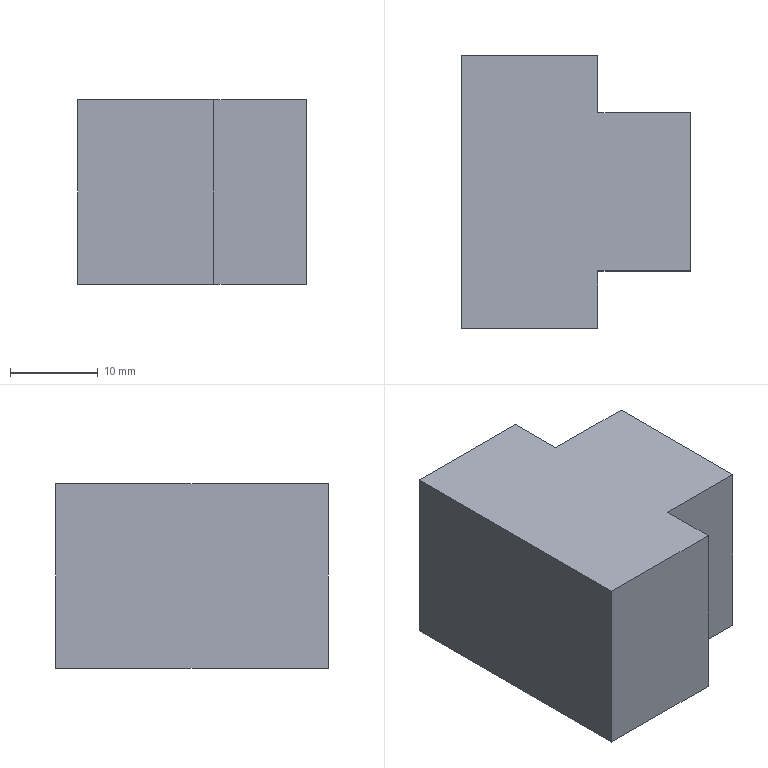Part | STEP file | PN_0024 | 1 solid | 13 faces | box 26 x 31 x 21 mm | volume 12363 mm3 | plane 11 | cylinder 2 | commonest cylinder face diameters 12 x2
STEP:
#1=CARTESIAN_POINT('',(0.,0.,0.));
#2=DIRECTION('',(0.,0.,1.));
#3=DIRECTION('',(1.,0.,0.));
#4=AXIS2_PLACEMENT_3D('',#1,#2,#3);
#5=CARTESIAN_POINT('',(11.,15.5,4.5));
#6=VERTEX_POINT('',#5);
#7=CARTESIAN_POINT('',(26.,15.5,4.5));
#8=VERTEX_POINT('',#7);
#9=CARTESIAN_POINT('',(11.,15.5,4.5));
#10=DIRECTION('',(1.,0.,0.));
#11=VECTOR('',#10,1.);
#12=LINE('',#9,#11);
#13=CARTESIAN_POINT('',(11.,15.5,10.5));
#14=DIRECTION('',(1.,0.,0.));
#15=DIRECTION('',(0.,0.,-1.));
#16=AXIS2_PLACEMENT_3D('',#13,#14,#15);
#17=CYLINDRICAL_SURFACE('',#16,6.);
#18=CARTESIAN_POINT('',(6.283,0.));
#19=DIRECTION('',(0.,1.));
#20=VECTOR('',#19,1.);
#21=LINE('',#18,#20);
#22=(GEOMETRIC_REPRESENTATION_CONTEXT(2)PARAMETRIC_REPRESENTATION_CONTEXT()REPRESENTATION_CONTEXT('',''));
#23=DEFINITIONAL_REPRESENTATION('',(#21),#22);
#24=PCURVE('',#17,#23);
#25=CARTESIAN_POINT('',(11.,15.5,10.5));
#26=DIRECTION('',(1.,0.,0.));
#27=DIRECTION('',(0.,0.,-1.));
#28=AXIS2_PLACEMENT_3D('',#25,#26,#27);
#29=CYLINDRICAL_SURFACE('',#28,6.);
#30=CARTESIAN_POINT('',(0.,0.));
#31=DIRECTION('',(0.,1.));
#32=VECTOR('',#31,1.);
#33=LINE('',#30,#32);
#34=(GEOMETRIC_REPRESENTATION_CONTEXT(2)PARAMETRIC_REPRESENTATION_CONTEXT()REPRESENTATION_CONTEXT('',''));
#35=DEFINITIONAL_REPRESENTATION('',(#33),#34);
#36=PCURVE('',#29,#35);
#37=SURFACE_CURVE('',#12,(#24,#36),.PCURVE_S1.);
#38=EDGE_CURVE('',#6,#8,#37,.T.);
#39=ORIENTED_EDGE('',*,*,#38,.T.);
#40=CARTESIAN_POINT('',(26.,15.5,16.5));
#41=VERTEX_POINT('',#40);
#42=CARTESIAN_POINT('',(26.,15.5,10.5));
#43=DIRECTION('',(1.,0.,0.));
#44=DIRECTION('',(0.,0.,-1.));
#45=AXIS2_PLACEMENT_3D('',#42,#43,#44);
#46=CIRCLE('',#45,6.);
#47=CARTESIAN_POINT('',(0.,15.));
#48=DIRECTION('',(1.,0.));
#49=VECTOR('',#48,1.);
#50=LINE('',#47,#49);
#51=(GEOMETRIC_REPRESENTATION_CONTEXT(2)PARAMETRIC_REPRESENTATION_CONTEXT()REPRESENTATION_CONTEXT('',''));
#52=DEFINITIONAL_REPRESENTATION('',(#50),#51);
#53=PCURVE('',#17,#52);
#54=CARTESIAN_POINT('',(26.,6.5,21.));
#55=DIRECTION('',(-1.,0.,0.));
#56=DIRECTION('',(0.,0.,1.));
#57=AXIS2_PLACEMENT_3D('',#54,#55,#56);
#58=PLANE('',#57);
#59=CARTESIAN_POINT('',(-16.5,9.));
#60=CARTESIAN_POINT('',(-16.5,19.392));
#61=CARTESIAN_POINT('',(-7.5,14.196));
#62=CARTESIAN_POINT('',(1.5,9.));
#63=CARTESIAN_POINT('',(-7.5,3.804));
#64=CARTESIAN_POINT('',(-16.5,-1.392));
#65=CARTESIAN_POINT('',(-16.5,9.));
#66=(BOUNDED_CURVE()B_SPLINE_CURVE(2,(#59,#60,#61,#62,#63,#64,#65),.UNSPECIFIED.,.T.,.F.)B_SPLINE_CURVE_WITH_KNOTS((1,2,2,2,2,1),(-2.094,0.,2.094,4.189,6.283,8.378),.UNSPECIFIED.)CURVE()GEOMETRIC_REPRESENTATION_ITEM()RATIONAL_B_SPLINE_CURVE((1.,0.5,1.,0.5,1.,0.5,1.))REPRESENTATION_ITEM(''));
#67=(GEOMETRIC_REPRESENTATION_CONTEXT(2)PARAMETRIC_REPRESENTATION_CONTEXT()REPRESENTATION_CONTEXT('',''));
#68=DEFINITIONAL_REPRESENTATION('',(#66),#67);
#69=PCURVE('',#58,#68);
#70=SURFACE_CURVE('',#46,(#53,#69),.PCURVE_S1.);
#71=EDGE_CURVE('',#41,#8,#70,.T.);
#72=ORIENTED_EDGE('',*,*,#71,.F.);
#73=CARTESIAN_POINT('',(11.,15.5,16.5));
#74=VERTEX_POINT('',#73);
#75=CARTESIAN_POINT('',(11.,15.5,16.5));
#76=DIRECTION('',(1.,0.,0.));
#77=VECTOR('',#76,1.);
#78=LINE('',#75,#77);
#79=CARTESIAN_POINT('',(3.142,0.));
#80=DIRECTION('',(0.,1.));
#81=VECTOR('',#80,1.);
#82=LINE('',#79,#81);
#83=(GEOMETRIC_REPRESENTATION_CONTEXT(2)PARAMETRIC_REPRESENTATION_CONTEXT()REPRESENTATION_CONTEXT('',''));
#84=DEFINITIONAL_REPRESENTATION('',(#82),#83);
#85=PCURVE('',#17,#84);
#86=CARTESIAN_POINT('',(3.142,0.));
#87=DIRECTION('',(0.,1.));
#88=VECTOR('',#87,1.);
#89=LINE('',#86,#88);
#90=(GEOMETRIC_REPRESENTATION_CONTEXT(2)PARAMETRIC_REPRESENTATION_CONTEXT()REPRESENTATION_CONTEXT('',''));
#91=DEFINITIONAL_REPRESENTATION('',(#89),#90);
#92=PCURVE('',#29,#91);
#93=SURFACE_CURVE('',#78,(#85,#92),.PCURVE_S1.);
#94=EDGE_CURVE('',#74,#41,#93,.T.);
#95=ORIENTED_EDGE('',*,*,#94,.F.);
#96=CARTESIAN_POINT('',(11.,15.5,10.5));
#97=DIRECTION('',(1.,0.,0.));
#98=DIRECTION('',(0.,0.,-1.));
#99=AXIS2_PLACEMENT_3D('',#96,#97,#98);
#100=CIRCLE('',#99,6.);
#101=CARTESIAN_POINT('',(0.,0.));
#102=DIRECTION('',(1.,0.));
#103=VECTOR('',#102,1.);
#104=LINE('',#101,#103);
#105=(GEOMETRIC_REPRESENTATION_CONTEXT(2)PARAMETRIC_REPRESENTATION_CONTEXT()REPRESENTATION_CONTEXT('',''));
#106=DEFINITIONAL_REPRESENTATION('',(#104),#105);
#107=PCURVE('',#17,#106);
#108=CARTESIAN_POINT('',(11.,15.5,10.5));
#109=DIRECTION('',(1.,0.,0.));
#110=DIRECTION('',(0.,0.,-1.));
#111=AXIS2_PLACEMENT_3D('',#108,#109,#110);
#112=PLANE('',#111);
#113=CARTESIAN_POINT('',(0.,0.));
#114=DIRECTION('',(1.,0.));
#115=AXIS2_PLACEMENT_2D('',#113,#114);
#116=CIRCLE('',#115,6.);
#117=(GEOMETRIC_REPRESENTATION_CONTEXT(2)PARAMETRIC_REPRESENTATION_CONTEXT()REPRESENTATION_CONTEXT('',''));
#118=DEFINITIONAL_REPRESENTATION('',(#116),#117);
#119=PCURVE('',#112,#118);
#120=SURFACE_CURVE('',#100,(#107,#119),.PCURVE_S1.);
#121=EDGE_CURVE('',#74,#6,#120,.T.);
#122=ORIENTED_EDGE('',*,*,#121,.T.);
#123=EDGE_LOOP('',(#39,#72,#95,#122));
#124=FACE_BOUND('',#123,.F.);
#125=ADVANCED_FACE('',(#124),#17,.F.);
#126=CARTESIAN_POINT('',(0.,31.,0.));
#127=VERTEX_POINT('',#126);
#128=CARTESIAN_POINT('',(0.,0.,0.));
#129=VERTEX_POINT('',#128);
#130=CARTESIAN_POINT('',(0.,0.,0.));
#131=DIRECTION('',(0.,-1.,0.));
#132=VECTOR('',#131,1.);
#133=LINE('',#130,#132);
#134=CARTESIAN_POINT('',(0.,0.,21.));
#135=DIRECTION('',(1.,0.,0.));
#136=DIRECTION('',(0.,0.,-1.));
#137=AXIS2_PLACEMENT_3D('',#134,#135,#136);
#138=PLANE('',#137);
#139=CARTESIAN_POINT('',(21.,0.));
#140=DIRECTION('',(0.,-1.));
#141=VECTOR('',#140,1.);
#142=LINE('',#139,#141);
#143=(GEOMETRIC_REPRESENTATION_CONTEXT(2)PARAMETRIC_REPRESENTATION_CONTEXT()REPRESENTATION_CONTEXT('',''));
#144=DEFINITIONAL_REPRESENTATION('',(#142),#143);
#145=PCURVE('',#138,#144);
#146=CARTESIAN_POINT('',(0.,31.,0.));
#147=DIRECTION('',(0.,0.,-1.));
#148=DIRECTION('',(-1.,0.,0.));
#149=AXIS2_PLACEMENT_3D('',#146,#147,#148);
#150=PLANE('',#149);
#151=CARTESIAN_POINT('',(0.,-31.));
#152=DIRECTION('',(0.,-1.));
#153=VECTOR('',#152,1.);
#154=LINE('',#151,#153);
#155=(GEOMETRIC_REPRESENTATION_CONTEXT(2)PARAMETRIC_REPRESENTATION_CONTEXT()REPRESENTATION_CONTEXT('',''));
#156=DEFINITIONAL_REPRESENTATION('',(#154),#155);
#157=PCURVE('',#150,#156);
#158=SURFACE_CURVE('',#133,(#145,#157),.PCURVE_S1.);
#159=EDGE_CURVE('',#127,#129,#158,.T.);
#160=ORIENTED_EDGE('',*,*,#159,.T.);
#161=CARTESIAN_POINT('',(0.,0.,21.));
#162=VERTEX_POINT('',#161);
#163=CARTESIAN_POINT('',(0.,0.,21.));
#164=DIRECTION('',(0.,0.,-1.));
#165=VECTOR('',#164,1.);
#166=LINE('',#163,#165);
#167=CARTESIAN_POINT('',(0.,0.));
#168=DIRECTION('',(1.,0.));
#169=VECTOR('',#168,1.);
#170=LINE('',#167,#169);
#171=(GEOMETRIC_REPRESENTATION_CONTEXT(2)PARAMETRIC_REPRESENTATION_CONTEXT()REPRESENTATION_CONTEXT('',''));
#172=DEFINITIONAL_REPRESENTATION('',(#170),#171);
#173=PCURVE('',#138,#172);
#174=CARTESIAN_POINT('',(0.,0.,21.));
#175=DIRECTION('',(0.,1.,0.));
#176=DIRECTION('',(0.,0.,1.));
#177=AXIS2_PLACEMENT_3D('',#174,#175,#176);
#178=PLANE('',#177);
#179=CARTESIAN_POINT('',(0.,0.));
#180=DIRECTION('',(-1.,0.));
#181=VECTOR('',#180,1.);
#182=LINE('',#179,#181);
#183=(GEOMETRIC_REPRESENTATION_CONTEXT(2)PARAMETRIC_REPRESENTATION_CONTEXT()REPRESENTATION_CONTEXT('',''));
#184=DEFINITIONAL_REPRESENTATION('',(#182),#183);
#185=PCURVE('',#178,#184);
#186=SURFACE_CURVE('',#166,(#173,#185),.PCURVE_S1.);
#187=EDGE_CURVE('',#162,#129,#186,.T.);
#188=ORIENTED_EDGE('',*,*,#187,.F.);
#189=CARTESIAN_POINT('',(0.,31.,21.));
#190=VERTEX_POINT('',#189);
#191=CARTESIAN_POINT('',(0.,0.,21.));
#192=DIRECTION('',(0.,-1.,0.));
#193=VECTOR('',#192,1.);
#194=LINE('',#191,#193);
#195=CARTESIAN_POINT('',(0.,0.));
#196=DIRECTION('',(0.,-1.));
#197=VECTOR('',#196,1.);
#198=LINE('',#195,#197);
#199=(GEOMETRIC_REPRESENTATION_CONTEXT(2)PARAMETRIC_REPRESENTATION_CONTEXT()REPRESENTATION_CONTEXT('',''));
#200=DEFINITIONAL_REPRESENTATION('',(#198),#199);
#201=PCURVE('',#138,#200);
#202=CARTESIAN_POINT('',(0.,31.,21.));
#203=DIRECTION('',(0.,0.,-1.));
#204=DIRECTION('',(-1.,0.,0.));
#205=AXIS2_PLACEMENT_3D('',#202,#203,#204);
#206=PLANE('',#205);
#207=CARTESIAN_POINT('',(0.,-31.));
#208=DIRECTION('',(0.,-1.));
#209=VECTOR('',#208,1.);
#210=LINE('',#207,#209);
#211=(GEOMETRIC_REPRESENTATION_CONTEXT(2)PARAMETRIC_REPRESENTATION_CONTEXT()REPRESENTATION_CONTEXT('',''));
#212=DEFINITIONAL_REPRESENTATION('',(#210),#211);
#213=PCURVE('',#206,#212);
#214=SURFACE_CURVE('',#194,(#201,#213),.PCURVE_S1.);
#215=EDGE_CURVE('',#190,#162,#214,.T.);
#216=ORIENTED_EDGE('',*,*,#215,.F.);
#217=CARTESIAN_POINT('',(0.,31.,21.));
#218=DIRECTION('',(0.,0.,-1.));
#219=VECTOR('',#218,1.);
#220=LINE('',#217,#219);
#221=CARTESIAN_POINT('',(0.,31.));
#222=DIRECTION('',(1.,0.));
#223=VECTOR('',#222,1.);
#224=LINE('',#221,#223);
#225=(GEOMETRIC_REPRESENTATION_CONTEXT(2)PARAMETRIC_REPRESENTATION_CONTEXT()REPRESENTATION_CONTEXT('',''));
#226=DEFINITIONAL_REPRESENTATION('',(#224),#225);
#227=PCURVE('',#138,#226);
#228=CARTESIAN_POINT('',(0.,31.,21.));
#229=DIRECTION('',(0.,-1.,0.));
#230=DIRECTION('',(0.,0.,-1.));
#231=AXIS2_PLACEMENT_3D('',#228,#229,#230);
#232=PLANE('',#231);
#233=CARTESIAN_POINT('',(0.,0.));
#234=DIRECTION('',(1.,0.));
#235=VECTOR('',#234,1.);
#236=LINE('',#233,#235);
#237=(GEOMETRIC_REPRESENTATION_CONTEXT(2)PARAMETRIC_REPRESENTATION_CONTEXT()REPRESENTATION_CONTEXT('',''));
#238=DEFINITIONAL_REPRESENTATION('',(#236),#237);
#239=PCURVE('',#232,#238);
#240=SURFACE_CURVE('',#220,(#227,#239),.PCURVE_S1.);
#241=EDGE_CURVE('',#190,#127,#240,.T.);
#242=ORIENTED_EDGE('',*,*,#241,.T.);
#243=EDGE_LOOP('',(#160,#188,#216,#242));
#244=FACE_BOUND('',#243,.T.);
#245=ADVANCED_FACE('',(#244),#138,.F.);
#246=CARTESIAN_POINT('',(15.5,0.,0.));
#247=VERTEX_POINT('',#246);
#248=CARTESIAN_POINT('',(0.,0.,0.));
#249=DIRECTION('',(1.,0.,0.));
#250=VECTOR('',#249,1.);
#251=LINE('',#248,#250);
#252=CARTESIAN_POINT('',(-21.,0.));
#253=DIRECTION('',(0.,1.));
#254=VECTOR('',#253,1.);
#255=LINE('',#252,#254);
#256=(GEOMETRIC_REPRESENTATION_CONTEXT(2)PARAMETRIC_REPRESENTATION_CONTEXT()REPRESENTATION_CONTEXT('',''));
#257=DEFINITIONAL_REPRESENTATION('',(#255),#256);
#258=PCURVE('',#178,#257);
#259=CARTESIAN_POINT('',(0.,-31.));
#260=DIRECTION('',(-1.,0.));
#261=VECTOR('',#260,1.);
#262=LINE('',#259,#261);
#263=(GEOMETRIC_REPRESENTATION_CONTEXT(2)PARAMETRIC_REPRESENTATION_CONTEXT()REPRESENTATION_CONTEXT('',''));
#264=DEFINITIONAL_REPRESENTATION('',(#262),#263);
#265=PCURVE('',#150,#264);
#266=SURFACE_CURVE('',#251,(#258,#265),.PCURVE_S1.);
#267=EDGE_CURVE('',#129,#247,#266,.T.);
#268=ORIENTED_EDGE('',*,*,#267,.T.);
#269=CARTESIAN_POINT('',(15.5,0.,21.));
#270=VERTEX_POINT('',#269);
#271=CARTESIAN_POINT('',(15.5,0.,21.));
#272=DIRECTION('',(0.,0.,-1.));
#273=VECTOR('',#272,1.);
#274=LINE('',#271,#273);
#275=CARTESIAN_POINT('',(0.,15.5));
#276=DIRECTION('',(-1.,0.));
#277=VECTOR('',#276,1.);
#278=LINE('',#275,#277);
#279=(GEOMETRIC_REPRESENTATION_CONTEXT(2)PARAMETRIC_REPRESENTATION_CONTEXT()REPRESENTATION_CONTEXT('',''));
#280=DEFINITIONAL_REPRESENTATION('',(#278),#279);
#281=PCURVE('',#178,#280);
#282=CARTESIAN_POINT('',(15.5,0.,21.));
#283=DIRECTION('',(-1.,0.,0.));
#284=DIRECTION('',(0.,0.,1.));
#285=AXIS2_PLACEMENT_3D('',#282,#283,#284);
#286=PLANE('',#285);
#287=CARTESIAN_POINT('',(0.,0.));
#288=DIRECTION('',(-1.,0.));
#289=VECTOR('',#288,1.);
#290=LINE('',#287,#289);
#291=(GEOMETRIC_REPRESENTATION_CONTEXT(2)PARAMETRIC_REPRESENTATION_CONTEXT()REPRESENTATION_CONTEXT('',''));
#292=DEFINITIONAL_REPRESENTATION('',(#290),#291);
#293=PCURVE('',#286,#292);
#294=SURFACE_CURVE('',#274,(#281,#293),.PCURVE_S1.);
#295=EDGE_CURVE('',#270,#247,#294,.T.);
#296=ORIENTED_EDGE('',*,*,#295,.F.);
#297=CARTESIAN_POINT('',(0.,0.,21.));
#298=DIRECTION('',(1.,0.,0.));
#299=VECTOR('',#298,1.);
#300=LINE('',#297,#299);
#301=CARTESIAN_POINT('',(0.,0.));
#302=DIRECTION('',(0.,1.));
#303=VECTOR('',#302,1.);
#304=LINE('',#301,#303);
#305=(GEOMETRIC_REPRESENTATION_CONTEXT(2)PARAMETRIC_REPRESENTATION_CONTEXT()REPRESENTATION_CONTEXT('',''));
#306=DEFINITIONAL_REPRESENTATION('',(#304),#305);
#307=PCURVE('',#178,#306);
#308=CARTESIAN_POINT('',(0.,-31.));
#309=DIRECTION('',(-1.,0.));
#310=VECTOR('',#309,1.);
#311=LINE('',#308,#310);
#312=(GEOMETRIC_REPRESENTATION_CONTEXT(2)PARAMETRIC_REPRESENTATION_CONTEXT()REPRESENTATION_CONTEXT('',''));
#313=DEFINITIONAL_REPRESENTATION('',(#311),#312);
#314=PCURVE('',#206,#313);
#315=SURFACE_CURVE('',#300,(#307,#314),.PCURVE_S1.);
#316=EDGE_CURVE('',#162,#270,#315,.T.);
#317=ORIENTED_EDGE('',*,*,#316,.F.);
#318=ORIENTED_EDGE('',*,*,#187,.T.);
#319=EDGE_LOOP('',(#268,#296,#317,#318));
#320=FACE_BOUND('',#319,.T.);
#321=ADVANCED_FACE('',(#320),#178,.F.);
#322=CARTESIAN_POINT('',(15.5,6.5,0.));
#323=VERTEX_POINT('',#322);
#324=CARTESIAN_POINT('',(15.5,0.,0.));
#325=DIRECTION('',(0.,1.,0.));
#326=VECTOR('',#325,1.);
#327=LINE('',#324,#326);
#328=CARTESIAN_POINT('',(-21.,0.));
#329=DIRECTION('',(0.,1.));
#330=VECTOR('',#329,1.);
#331=LINE('',#328,#330);
#332=(GEOMETRIC_REPRESENTATION_CONTEXT(2)PARAMETRIC_REPRESENTATION_CONTEXT()REPRESENTATION_CONTEXT('',''));
#333=DEFINITIONAL_REPRESENTATION('',(#331),#332);
#334=PCURVE('',#286,#333);
#335=CARTESIAN_POINT('',(-15.5,-31.));
#336=DIRECTION('',(0.,1.));
#337=VECTOR('',#336,1.);
#338=LINE('',#335,#337);
#339=(GEOMETRIC_REPRESENTATION_CONTEXT(2)PARAMETRIC_REPRESENTATION_CONTEXT()REPRESENTATION_CONTEXT('',''));
#340=DEFINITIONAL_REPRESENTATION('',(#338),#339);
#341=PCURVE('',#150,#340);
#342=SURFACE_CURVE('',#327,(#334,#341),.PCURVE_S1.);
#343=EDGE_CURVE('',#247,#323,#342,.T.);
#344=ORIENTED_EDGE('',*,*,#343,.T.);
#345=CARTESIAN_POINT('',(15.5,6.5,21.));
#346=VERTEX_POINT('',#345);
#347=CARTESIAN_POINT('',(15.5,6.5,21.));
#348=DIRECTION('',(0.,0.,-1.));
#349=VECTOR('',#348,1.);
#350=LINE('',#347,#349);
#351=CARTESIAN_POINT('',(0.,6.5));
#352=DIRECTION('',(-1.,0.));
#353=VECTOR('',#352,1.);
#354=LINE('',#351,#353);
#355=(GEOMETRIC_REPRESENTATION_CONTEXT(2)PARAMETRIC_REPRESENTATION_CONTEXT()REPRESENTATION_CONTEXT('',''));
#356=DEFINITIONAL_REPRESENTATION('',(#354),#355);
#357=PCURVE('',#286,#356);
#358=CARTESIAN_POINT('',(15.5,6.5,21.));
#359=DIRECTION('',(0.,1.,0.));
#360=DIRECTION('',(0.,0.,1.));
#361=AXIS2_PLACEMENT_3D('',#358,#359,#360);
#362=PLANE('',#361);
#363=CARTESIAN_POINT('',(0.,0.));
#364=DIRECTION('',(-1.,0.));
#365=VECTOR('',#364,1.);
#366=LINE('',#363,#365);
#367=(GEOMETRIC_REPRESENTATION_CONTEXT(2)PARAMETRIC_REPRESENTATION_CONTEXT()REPRESENTATION_CONTEXT('',''));
#368=DEFINITIONAL_REPRESENTATION('',(#366),#367);
#369=PCURVE('',#362,#368);
#370=SURFACE_CURVE('',#350,(#357,#369),.PCURVE_S1.);
#371=EDGE_CURVE('',#346,#323,#370,.T.);
#372=ORIENTED_EDGE('',*,*,#371,.F.);
#373=CARTESIAN_POINT('',(15.5,0.,21.));
#374=DIRECTION('',(0.,1.,0.));
#375=VECTOR('',#374,1.);
#376=LINE('',#373,#375);
#377=CARTESIAN_POINT('',(0.,0.));
#378=DIRECTION('',(0.,1.));
#379=VECTOR('',#378,1.);
#380=LINE('',#377,#379);
#381=(GEOMETRIC_REPRESENTATION_CONTEXT(2)PARAMETRIC_REPRESENTATION_CONTEXT()REPRESENTATION_CONTEXT('',''));
#382=DEFINITIONAL_REPRESENTATION('',(#380),#381);
#383=PCURVE('',#286,#382);
#384=CARTESIAN_POINT('',(-15.5,-31.));
#385=DIRECTION('',(0.,1.));
#386=VECTOR('',#385,1.);
#387=LINE('',#384,#386);
#388=(GEOMETRIC_REPRESENTATION_CONTEXT(2)PARAMETRIC_REPRESENTATION_CONTEXT()REPRESENTATION_CONTEXT('',''));
#389=DEFINITIONAL_REPRESENTATION('',(#387),#388);
#390=PCURVE('',#206,#389);
#391=SURFACE_CURVE('',#376,(#383,#390),.PCURVE_S1.);
#392=EDGE_CURVE('',#270,#346,#391,.T.);
#393=ORIENTED_EDGE('',*,*,#392,.F.);
#394=ORIENTED_EDGE('',*,*,#295,.T.);
#395=EDGE_LOOP('',(#344,#372,#393,#394));
#396=FACE_BOUND('',#395,.T.);
#397=ADVANCED_FACE('',(#396),#286,.F.);
#398=CARTESIAN_POINT('',(26.,6.5,0.));
#399=VERTEX_POINT('',#398);
#400=CARTESIAN_POINT('',(15.5,6.5,0.));
#401=DIRECTION('',(1.,0.,0.));
#402=VECTOR('',#401,1.);
#403=LINE('',#400,#402);
#404=CARTESIAN_POINT('',(-21.,0.));
#405=DIRECTION('',(0.,1.));
#406=VECTOR('',#405,1.);
#407=LINE('',#404,#406);
#408=(GEOMETRIC_REPRESENTATION_CONTEXT(2)PARAMETRIC_REPRESENTATION_CONTEXT()REPRESENTATION_CONTEXT('',''));
#409=DEFINITIONAL_REPRESENTATION('',(#407),#408);
#410=PCURVE('',#362,#409);
#411=CARTESIAN_POINT('',(-15.5,-24.5));
#412=DIRECTION('',(-1.,0.));
#413=VECTOR('',#412,1.);
#414=LINE('',#411,#413);
#415=(GEOMETRIC_REPRESENTATION_CONTEXT(2)PARAMETRIC_REPRESENTATION_CONTEXT()REPRESENTATION_CONTEXT('',''));
#416=DEFINITIONAL_REPRESENTATION('',(#414),#415);
#417=PCURVE('',#150,#416);
#418=SURFACE_CURVE('',#403,(#410,#417),.PCURVE_S1.);
#419=EDGE_CURVE('',#323,#399,#418,.T.);
#420=ORIENTED_EDGE('',*,*,#419,.T.);
#421=CARTESIAN_POINT('',(26.,6.5,21.));
#422=VERTEX_POINT('',#421);
#423=CARTESIAN_POINT('',(26.,6.5,21.));
#424=DIRECTION('',(0.,0.,-1.));
#425=VECTOR('',#424,1.);
#426=LINE('',#423,#425);
#427=CARTESIAN_POINT('',(0.,10.5));
#428=DIRECTION('',(-1.,0.));
#429=VECTOR('',#428,1.);
#430=LINE('',#427,#429);
#431=(GEOMETRIC_REPRESENTATION_CONTEXT(2)PARAMETRIC_REPRESENTATION_CONTEXT()REPRESENTATION_CONTEXT('',''));
#432=DEFINITIONAL_REPRESENTATION('',(#430),#431);
#433=PCURVE('',#362,#432);
#434=CARTESIAN_POINT('',(0.,0.));
#435=DIRECTION('',(-1.,0.));
#436=VECTOR('',#435,1.);
#437=LINE('',#434,#436);
#438=(GEOMETRIC_REPRESENTATION_CONTEXT(2)PARAMETRIC_REPRESENTATION_CONTEXT()REPRESENTATION_CONTEXT('',''));
#439=DEFINITIONAL_REPRESENTATION('',(#437),#438);
#440=PCURVE('',#58,#439);
#441=SURFACE_CURVE('',#426,(#433,#440),.PCURVE_S1.);
#442=EDGE_CURVE('',#422,#399,#441,.T.);
#443=ORIENTED_EDGE('',*,*,#442,.F.);
#444=CARTESIAN_POINT('',(15.5,6.5,21.));
#445=DIRECTION('',(1.,0.,0.));
#446=VECTOR('',#445,1.);
#447=LINE('',#444,#446);
#448=CARTESIAN_POINT('',(0.,0.));
#449=DIRECTION('',(0.,1.));
#450=VECTOR('',#449,1.);
#451=LINE('',#448,#450);
#452=(GEOMETRIC_REPRESENTATION_CONTEXT(2)PARAMETRIC_REPRESENTATION_CONTEXT()REPRESENTATION_CONTEXT('',''));
#453=DEFINITIONAL_REPRESENTATION('',(#451),#452);
#454=PCURVE('',#362,#453);
#455=CARTESIAN_POINT('',(-15.5,-24.5));
#456=DIRECTION('',(-1.,0.));
#457=VECTOR('',#456,1.);
#458=LINE('',#455,#457);
#459=(GEOMETRIC_REPRESENTATION_CONTEXT(2)PARAMETRIC_REPRESENTATION_CONTEXT()REPRESENTATION_CONTEXT('',''));
#460=DEFINITIONAL_REPRESENTATION('',(#458),#459);
#461=PCURVE('',#206,#460);
#462=SURFACE_CURVE('',#447,(#454,#461),.PCURVE_S1.);
#463=EDGE_CURVE('',#346,#422,#462,.T.);
#464=ORIENTED_EDGE('',*,*,#463,.F.);
#465=ORIENTED_EDGE('',*,*,#371,.T.);
#466=EDGE_LOOP('',(#420,#443,#464,#465));
#467=FACE_BOUND('',#466,.T.);
#468=ADVANCED_FACE('',(#467),#362,.F.);
#469=CARTESIAN_POINT('',(26.,15.5,10.5));
#470=DIRECTION('',(1.,0.,0.));
#471=DIRECTION('',(0.,0.,-1.));
#472=AXIS2_PLACEMENT_3D('',#469,#470,#471);
#473=CIRCLE('',#472,6.);
#474=CARTESIAN_POINT('',(-16.5,9.));
#475=CARTESIAN_POINT('',(-16.5,19.392));
#476=CARTESIAN_POINT('',(-7.5,14.196));
#477=CARTESIAN_POINT('',(1.5,9.));
#478=CARTESIAN_POINT('',(-7.5,3.804));
#479=CARTESIAN_POINT('',(-16.5,-1.392));
#480=CARTESIAN_POINT('',(-16.5,9.));
#481=(BOUNDED_CURVE()B_SPLINE_CURVE(2,(#474,#475,#476,#477,#478,#479,#480),.UNSPECIFIED.,.T.,.F.)B_SPLINE_CURVE_WITH_KNOTS((1,2,2,2,2,1),(-2.094,0.,2.094,4.189,6.283,8.378),.UNSPECIFIED.)CURVE()GEOMETRIC_REPRESENTATION_ITEM()RATIONAL_B_SPLINE_CURVE((1.,0.5,1.,0.5,1.,0.5,1.))REPRESENTATION_ITEM(''));
#482=(GEOMETRIC_REPRESENTATION_CONTEXT(2)PARAMETRIC_REPRESENTATION_CONTEXT()REPRESENTATION_CONTEXT('',''));
#483=DEFINITIONAL_REPRESENTATION('',(#481),#482);
#484=PCURVE('',#58,#483);
#485=CARTESIAN_POINT('',(0.,15.));
#486=DIRECTION('',(1.,0.));
#487=VECTOR('',#486,1.);
#488=LINE('',#485,#487);
#489=(GEOMETRIC_REPRESENTATION_CONTEXT(2)PARAMETRIC_REPRESENTATION_CONTEXT()REPRESENTATION_CONTEXT('',''));
#490=DEFINITIONAL_REPRESENTATION('',(#488),#489);
#491=PCURVE('',#29,#490);
#492=SURFACE_CURVE('',#473,(#484,#491),.PCURVE_S1.);
#493=EDGE_CURVE('',#8,#41,#492,.T.);
#494=ORIENTED_EDGE('',*,*,#493,.F.);
#495=ORIENTED_EDGE('',*,*,#71,.F.);
#496=EDGE_LOOP('',(#494,#495));
#497=FACE_BOUND('',#496,.T.);
#498=CARTESIAN_POINT('',(26.,24.5,0.));
#499=VERTEX_POINT('',#498);
#500=CARTESIAN_POINT('',(26.,6.5,0.));
#501=DIRECTION('',(0.,1.,0.));
#502=VECTOR('',#501,1.);
#503=LINE('',#500,#502);
#504=CARTESIAN_POINT('',(-21.,0.));
#505=DIRECTION('',(0.,1.));
#506=VECTOR('',#505,1.);
#507=LINE('',#504,#506);
#508=(GEOMETRIC_REPRESENTATION_CONTEXT(2)PARAMETRIC_REPRESENTATION_CONTEXT()REPRESENTATION_CONTEXT('',''));
#509=DEFINITIONAL_REPRESENTATION('',(#507),#508);
#510=PCURVE('',#58,#509);
#511=CARTESIAN_POINT('',(-26.,-24.5));
#512=DIRECTION('',(0.,1.));
#513=VECTOR('',#512,1.);
#514=LINE('',#511,#513);
#515=(GEOMETRIC_REPRESENTATION_CONTEXT(2)PARAMETRIC_REPRESENTATION_CONTEXT()REPRESENTATION_CONTEXT('',''));
#516=DEFINITIONAL_REPRESENTATION('',(#514),#515);
#517=PCURVE('',#150,#516);
#518=SURFACE_CURVE('',#503,(#510,#517),.PCURVE_S1.);
#519=EDGE_CURVE('',#399,#499,#518,.T.);
#520=ORIENTED_EDGE('',*,*,#519,.T.);
#521=CARTESIAN_POINT('',(26.,24.5,21.));
#522=VERTEX_POINT('',#521);
#523=CARTESIAN_POINT('',(26.,24.5,21.));
#524=DIRECTION('',(0.,0.,-1.));
#525=VECTOR('',#524,1.);
#526=LINE('',#523,#525);
#527=CARTESIAN_POINT('',(0.,18.));
#528=DIRECTION('',(-1.,0.));
#529=VECTOR('',#528,1.);
#530=LINE('',#527,#529);
#531=(GEOMETRIC_REPRESENTATION_CONTEXT(2)PARAMETRIC_REPRESENTATION_CONTEXT()REPRESENTATION_CONTEXT('',''));
#532=DEFINITIONAL_REPRESENTATION('',(#530),#531);
#533=PCURVE('',#58,#532);
#534=CARTESIAN_POINT('',(15.5,24.5,21.));
#535=DIRECTION('',(0.,-1.,0.));
#536=DIRECTION('',(0.,0.,-1.));
#537=AXIS2_PLACEMENT_3D('',#534,#535,#536);
#538=PLANE('',#537);
#539=CARTESIAN_POINT('',(0.,10.5));
#540=DIRECTION('',(1.,0.));
#541=VECTOR('',#540,1.);
#542=LINE('',#539,#541);
#543=(GEOMETRIC_REPRESENTATION_CONTEXT(2)PARAMETRIC_REPRESENTATION_CONTEXT()REPRESENTATION_CONTEXT('',''));
#544=DEFINITIONAL_REPRESENTATION('',(#542),#543);
#545=PCURVE('',#538,#544);
#546=SURFACE_CURVE('',#526,(#533,#545),.PCURVE_S1.);
#547=EDGE_CURVE('',#522,#499,#546,.T.);
#548=ORIENTED_EDGE('',*,*,#547,.F.);
#549=CARTESIAN_POINT('',(26.,6.5,21.));
#550=DIRECTION('',(0.,1.,0.));
#551=VECTOR('',#550,1.);
#552=LINE('',#549,#551);
#553=CARTESIAN_POINT('',(0.,0.));
#554=DIRECTION('',(0.,1.));
#555=VECTOR('',#554,1.);
#556=LINE('',#553,#555);
#557=(GEOMETRIC_REPRESENTATION_CONTEXT(2)PARAMETRIC_REPRESENTATION_CONTEXT()REPRESENTATION_CONTEXT('',''));
#558=DEFINITIONAL_REPRESENTATION('',(#556),#557);
#559=PCURVE('',#58,#558);
#560=CARTESIAN_POINT('',(-26.,-24.5));
#561=DIRECTION('',(0.,1.));
#562=VECTOR('',#561,1.);
#563=LINE('',#560,#562);
#564=(GEOMETRIC_REPRESENTATION_CONTEXT(2)PARAMETRIC_REPRESENTATION_CONTEXT()REPRESENTATION_CONTEXT('',''));
#565=DEFINITIONAL_REPRESENTATION('',(#563),#564);
#566=PCURVE('',#206,#565);
#567=SURFACE_CURVE('',#552,(#559,#566),.PCURVE_S1.);
#568=EDGE_CURVE('',#422,#522,#567,.T.);
#569=ORIENTED_EDGE('',*,*,#568,.F.);
#570=ORIENTED_EDGE('',*,*,#442,.T.);
#571=EDGE_LOOP('',(#520,#548,#569,#570));
#572=FACE_BOUND('',#571,.T.);
#573=ADVANCED_FACE('',(#497,#572),#58,.F.);
#574=CARTESIAN_POINT('',(15.5,24.5,0.));
#575=VERTEX_POINT('',#574);
#576=CARTESIAN_POINT('',(15.5,24.5,0.));
#577=DIRECTION('',(-1.,0.,0.));
#578=VECTOR('',#577,1.);
#579=LINE('',#576,#578);
#580=CARTESIAN_POINT('',(21.,0.));
#581=DIRECTION('',(0.,-1.));
#582=VECTOR('',#581,1.);
#583=LINE('',#580,#582);
#584=(GEOMETRIC_REPRESENTATION_CONTEXT(2)PARAMETRIC_REPRESENTATION_CONTEXT()REPRESENTATION_CONTEXT('',''));
#585=DEFINITIONAL_REPRESENTATION('',(#583),#584);
#586=PCURVE('',#538,#585);
#587=CARTESIAN_POINT('',(-15.5,-6.5));
#588=DIRECTION('',(1.,0.));
#589=VECTOR('',#588,1.);
#590=LINE('',#587,#589);
#591=(GEOMETRIC_REPRESENTATION_CONTEXT(2)PARAMETRIC_REPRESENTATION_CONTEXT()REPRESENTATION_CONTEXT('',''));
#592=DEFINITIONAL_REPRESENTATION('',(#590),#591);
#593=PCURVE('',#150,#592);
#594=SURFACE_CURVE('',#579,(#586,#593),.PCURVE_S1.);
#595=EDGE_CURVE('',#499,#575,#594,.T.);
#596=ORIENTED_EDGE('',*,*,#595,.T.);
#597=CARTESIAN_POINT('',(15.5,24.5,21.));
#598=VERTEX_POINT('',#597);
#599=CARTESIAN_POINT('',(15.5,24.5,21.));
#600=DIRECTION('',(0.,0.,-1.));
#601=VECTOR('',#600,1.);
#602=LINE('',#599,#601);
#603=CARTESIAN_POINT('',(0.,0.));
#604=DIRECTION('',(1.,0.));
#605=VECTOR('',#604,1.);
#606=LINE('',#603,#605);
#607=(GEOMETRIC_REPRESENTATION_CONTEXT(2)PARAMETRIC_REPRESENTATION_CONTEXT()REPRESENTATION_CONTEXT('',''));
#608=DEFINITIONAL_REPRESENTATION('',(#606),#607);
#609=PCURVE('',#538,#608);
#610=CARTESIAN_POINT('',(15.5,24.5,21.));
#611=DIRECTION('',(-1.,0.,0.));
#612=DIRECTION('',(0.,0.,1.));
#613=AXIS2_PLACEMENT_3D('',#610,#611,#612);
#614=PLANE('',#613);
#615=CARTESIAN_POINT('',(0.,0.));
#616=DIRECTION('',(-1.,0.));
#617=VECTOR('',#616,1.);
#618=LINE('',#615,#617);
#619=(GEOMETRIC_REPRESENTATION_CONTEXT(2)PARAMETRIC_REPRESENTATION_CONTEXT()REPRESENTATION_CONTEXT('',''));
#620=DEFINITIONAL_REPRESENTATION('',(#618),#619);
#621=PCURVE('',#614,#620);
#622=SURFACE_CURVE('',#602,(#609,#621),.PCURVE_S1.);
#623=EDGE_CURVE('',#598,#575,#622,.T.);
#624=ORIENTED_EDGE('',*,*,#623,.F.);
#625=CARTESIAN_POINT('',(15.5,24.5,21.));
#626=DIRECTION('',(-1.,0.,0.));
#627=VECTOR('',#626,1.);
#628=LINE('',#625,#627);
#629=CARTESIAN_POINT('',(0.,0.));
#630=DIRECTION('',(0.,-1.));
#631=VECTOR('',#630,1.);
#632=LINE('',#629,#631);
#633=(GEOMETRIC_REPRESENTATION_CONTEXT(2)PARAMETRIC_REPRESENTATION_CONTEXT()REPRESENTATION_CONTEXT('',''));
#634=DEFINITIONAL_REPRESENTATION('',(#632),#633);
#635=PCURVE('',#538,#634);
#636=CARTESIAN_POINT('',(-15.5,-6.5));
#637=DIRECTION('',(1.,0.));
#638=VECTOR('',#637,1.);
#639=LINE('',#636,#638);
#640=(GEOMETRIC_REPRESENTATION_CONTEXT(2)PARAMETRIC_REPRESENTATION_CONTEXT()REPRESENTATION_CONTEXT('',''));
#641=DEFINITIONAL_REPRESENTATION('',(#639),#640);
#642=PCURVE('',#206,#641);
#643=SURFACE_CURVE('',#628,(#635,#642),.PCURVE_S1.);
#644=EDGE_CURVE('',#522,#598,#643,.T.);
#645=ORIENTED_EDGE('',*,*,#644,.F.);
#646=ORIENTED_EDGE('',*,*,#547,.T.);
#647=EDGE_LOOP('',(#596,#624,#645,#646));
#648=FACE_BOUND('',#647,.T.);
#649=ADVANCED_FACE('',(#648),#538,.F.);
#650=CARTESIAN_POINT('',(15.5,31.,0.));
#651=VERTEX_POINT('',#650);
#652=CARTESIAN_POINT('',(15.5,24.5,0.));
#653=DIRECTION('',(0.,1.,0.));
#654=VECTOR('',#653,1.);
#655=LINE('',#652,#654);
#656=CARTESIAN_POINT('',(-21.,0.));
#657=DIRECTION('',(0.,1.));
#658=VECTOR('',#657,1.);
#659=LINE('',#656,#658);
#660=(GEOMETRIC_REPRESENTATION_CONTEXT(2)PARAMETRIC_REPRESENTATION_CONTEXT()REPRESENTATION_CONTEXT('',''));
#661=DEFINITIONAL_REPRESENTATION('',(#659),#660);
#662=PCURVE('',#614,#661);
#663=CARTESIAN_POINT('',(-15.5,-6.5));
#664=DIRECTION('',(0.,1.));
#665=VECTOR('',#664,1.);
#666=LINE('',#663,#665);
#667=(GEOMETRIC_REPRESENTATION_CONTEXT(2)PARAMETRIC_REPRESENTATION_CONTEXT()REPRESENTATION_CONTEXT('',''));
#668=DEFINITIONAL_REPRESENTATION('',(#666),#667);
#669=PCURVE('',#150,#668);
#670=SURFACE_CURVE('',#655,(#662,#669),.PCURVE_S1.);
#671=EDGE_CURVE('',#575,#651,#670,.T.);
#672=ORIENTED_EDGE('',*,*,#671,.T.);
#673=CARTESIAN_POINT('',(15.5,31.,21.));
#674=VERTEX_POINT('',#673);
#675=CARTESIAN_POINT('',(15.5,31.,21.));
#676=DIRECTION('',(0.,0.,-1.));
#677=VECTOR('',#676,1.);
#678=LINE('',#675,#677);
#679=CARTESIAN_POINT('',(0.,6.5));
#680=DIRECTION('',(-1.,0.));
#681=VECTOR('',#680,1.);
#682=LINE('',#679,#681);
#683=(GEOMETRIC_REPRESENTATION_CONTEXT(2)PARAMETRIC_REPRESENTATION_CONTEXT()REPRESENTATION_CONTEXT('',''));
#684=DEFINITIONAL_REPRESENTATION('',(#682),#683);
#685=PCURVE('',#614,#684);
#686=CARTESIAN_POINT('',(0.,15.5));
#687=DIRECTION('',(1.,0.));
#688=VECTOR('',#687,1.);
#689=LINE('',#686,#688);
#690=(GEOMETRIC_REPRESENTATION_CONTEXT(2)PARAMETRIC_REPRESENTATION_CONTEXT()REPRESENTATION_CONTEXT('',''));
#691=DEFINITIONAL_REPRESENTATION('',(#689),#690);
#692=PCURVE('',#232,#691);
#693=SURFACE_CURVE('',#678,(#685,#692),.PCURVE_S1.);
#694=EDGE_CURVE('',#674,#651,#693,.T.);
#695=ORIENTED_EDGE('',*,*,#694,.F.);
#696=CARTESIAN_POINT('',(15.5,24.5,21.));
#697=DIRECTION('',(0.,1.,0.));
#698=VECTOR('',#697,1.);
#699=LINE('',#696,#698);
#700=CARTESIAN_POINT('',(0.,0.));
#701=DIRECTION('',(0.,1.));
#702=VECTOR('',#701,1.);
#703=LINE('',#700,#702);
#704=(GEOMETRIC_REPRESENTATION_CONTEXT(2)PARAMETRIC_REPRESENTATION_CONTEXT()REPRESENTATION_CONTEXT('',''));
#705=DEFINITIONAL_REPRESENTATION('',(#703),#704);
#706=PCURVE('',#614,#705);
#707=CARTESIAN_POINT('',(-15.5,-6.5));
#708=DIRECTION('',(0.,1.));
#709=VECTOR('',#708,1.);
#710=LINE('',#707,#709);
#711=(GEOMETRIC_REPRESENTATION_CONTEXT(2)PARAMETRIC_REPRESENTATION_CONTEXT()REPRESENTATION_CONTEXT('',''));
#712=DEFINITIONAL_REPRESENTATION('',(#710),#711);
#713=PCURVE('',#206,#712);
#714=SURFACE_CURVE('',#699,(#706,#713),.PCURVE_S1.);
#715=EDGE_CURVE('',#598,#674,#714,.T.);
#716=ORIENTED_EDGE('',*,*,#715,.F.);
#717=ORIENTED_EDGE('',*,*,#623,.T.);
#718=EDGE_LOOP('',(#672,#695,#716,#717));
#719=FACE_BOUND('',#718,.T.);
#720=ADVANCED_FACE('',(#719),#614,.F.);
#721=CARTESIAN_POINT('',(0.,31.,0.));
#722=DIRECTION('',(-1.,0.,0.));
#723=VECTOR('',#722,1.);
#724=LINE('',#721,#723);
#725=CARTESIAN_POINT('',(21.,0.));
#726=DIRECTION('',(0.,-1.));
#727=VECTOR('',#726,1.);
#728=LINE('',#725,#727);
#729=(GEOMETRIC_REPRESENTATION_CONTEXT(2)PARAMETRIC_REPRESENTATION_CONTEXT()REPRESENTATION_CONTEXT('',''));
#730=DEFINITIONAL_REPRESENTATION('',(#728),#729);
#731=PCURVE('',#232,#730);
#732=CARTESIAN_POINT('',(0.,0.));
#733=DIRECTION('',(1.,0.));
#734=VECTOR('',#733,1.);
#735=LINE('',#732,#734);
#736=(GEOMETRIC_REPRESENTATION_CONTEXT(2)PARAMETRIC_REPRESENTATION_CONTEXT()REPRESENTATION_CONTEXT('',''));
#737=DEFINITIONAL_REPRESENTATION('',(#735),#736);
#738=PCURVE('',#150,#737);
#739=SURFACE_CURVE('',#724,(#731,#738),.PCURVE_S1.);
#740=EDGE_CURVE('',#651,#127,#739,.T.);
#741=ORIENTED_EDGE('',*,*,#740,.T.);
#742=ORIENTED_EDGE('',*,*,#241,.F.);
#743=CARTESIAN_POINT('',(0.,31.,21.));
#744=DIRECTION('',(-1.,0.,0.));
#745=VECTOR('',#744,1.);
#746=LINE('',#743,#745);
#747=CARTESIAN_POINT('',(0.,0.));
#748=DIRECTION('',(0.,-1.));
#749=VECTOR('',#748,1.);
#750=LINE('',#747,#749);
#751=(GEOMETRIC_REPRESENTATION_CONTEXT(2)PARAMETRIC_REPRESENTATION_CONTEXT()REPRESENTATION_CONTEXT('',''));
#752=DEFINITIONAL_REPRESENTATION('',(#750),#751);
#753=PCURVE('',#232,#752);
#754=CARTESIAN_POINT('',(0.,0.));
#755=DIRECTION('',(1.,0.));
#756=VECTOR('',#755,1.);
#757=LINE('',#754,#756);
#758=(GEOMETRIC_REPRESENTATION_CONTEXT(2)PARAMETRIC_REPRESENTATION_CONTEXT()REPRESENTATION_CONTEXT('',''));
#759=DEFINITIONAL_REPRESENTATION('',(#757),#758);
#760=PCURVE('',#206,#759);
#761=SURFACE_CURVE('',#746,(#753,#760),.PCURVE_S1.);
#762=EDGE_CURVE('',#674,#190,#761,.T.);
#763=ORIENTED_EDGE('',*,*,#762,.F.);
#764=ORIENTED_EDGE('',*,*,#694,.T.);
#765=EDGE_LOOP('',(#741,#742,#763,#764));
#766=FACE_BOUND('',#765,.T.);
#767=ADVANCED_FACE('',(#766),#232,.F.);
#768=ORIENTED_EDGE('',*,*,#215,.T.);
#769=ORIENTED_EDGE('',*,*,#316,.T.);
#770=ORIENTED_EDGE('',*,*,#392,.T.);
#771=ORIENTED_EDGE('',*,*,#463,.T.);
#772=ORIENTED_EDGE('',*,*,#568,.T.);
#773=ORIENTED_EDGE('',*,*,#644,.T.);
#774=ORIENTED_EDGE('',*,*,#715,.T.);
#775=ORIENTED_EDGE('',*,*,#762,.T.);
#776=EDGE_LOOP('',(#768,#769,#770,#771,#772,#773,#774,#775));
#777=FACE_BOUND('',#776,.T.);
#778=ADVANCED_FACE('',(#777),#206,.F.);
#779=ORIENTED_EDGE('',*,*,#159,.F.);
#780=ORIENTED_EDGE('',*,*,#740,.F.);
#781=ORIENTED_EDGE('',*,*,#671,.F.);
#782=ORIENTED_EDGE('',*,*,#595,.F.);
#783=ORIENTED_EDGE('',*,*,#519,.F.);
#784=ORIENTED_EDGE('',*,*,#419,.F.);
#785=ORIENTED_EDGE('',*,*,#343,.F.);
#786=ORIENTED_EDGE('',*,*,#267,.F.);
#787=EDGE_LOOP('',(#779,#780,#781,#782,#783,#784,#785,#786));
#788=FACE_BOUND('',#787,.T.);
#789=ADVANCED_FACE('',(#788),#150,.T.);
#790=ORIENTED_EDGE('',*,*,#493,.F.);
#791=ORIENTED_EDGE('',*,*,#38,.F.);
#792=CARTESIAN_POINT('',(11.,15.5,10.5));
#793=DIRECTION('',(1.,0.,0.));
#794=DIRECTION('',(0.,0.,-1.));
#795=AXIS2_PLACEMENT_3D('',#792,#793,#794);
#796=CIRCLE('',#795,6.);
#797=CARTESIAN_POINT('',(0.,0.));
#798=DIRECTION('',(1.,0.));
#799=VECTOR('',#798,1.);
#800=LINE('',#797,#799);
#801=(GEOMETRIC_REPRESENTATION_CONTEXT(2)PARAMETRIC_REPRESENTATION_CONTEXT()REPRESENTATION_CONTEXT('',''));
#802=DEFINITIONAL_REPRESENTATION('',(#800),#801);
#803=PCURVE('',#29,#802);
#804=CARTESIAN_POINT('',(0.,0.));
#805=DIRECTION('',(1.,0.));
#806=AXIS2_PLACEMENT_2D('',#804,#805);
#807=CIRCLE('',#806,6.);
#808=(GEOMETRIC_REPRESENTATION_CONTEXT(2)PARAMETRIC_REPRESENTATION_CONTEXT()REPRESENTATION_CONTEXT('',''));
#809=DEFINITIONAL_REPRESENTATION('',(#807),#808);
#810=PCURVE('',#112,#809);
#811=SURFACE_CURVE('',#796,(#803,#810),.PCURVE_S1.);
#812=EDGE_CURVE('',#6,#74,#811,.T.);
#813=ORIENTED_EDGE('',*,*,#812,.T.);
#814=ORIENTED_EDGE('',*,*,#94,.T.);
#815=EDGE_LOOP('',(#790,#791,#813,#814));
#816=FACE_BOUND('',#815,.F.);
#817=ADVANCED_FACE('',(#816),#29,.F.);
#818=ORIENTED_EDGE('',*,*,#812,.T.);
#819=ORIENTED_EDGE('',*,*,#121,.T.);
#820=EDGE_LOOP('',(#818,#819));
#821=FACE_BOUND('',#820,.T.);
#822=ADVANCED_FACE('',(#821),#112,.T.);
#823=CLOSED_SHELL('',(#125,#245,#321,#397,#468,#573,#649,#720,#767,#778,#789,#817,#822));
#824=MANIFOLD_SOLID_BREP('',#823);
#825=(LENGTH_UNIT()NAMED_UNIT(*)SI_UNIT(.MILLI.,.METRE.));
#826=UNCERTAINTY_MEASURE_WITH_UNIT(LENGTH_MEASURE(0.0000001),#825,'','');
#827=(NAMED_UNIT(*)PLANE_ANGLE_UNIT()SI_UNIT($,.RADIAN.));
#828=(NAMED_UNIT(*)SI_UNIT($,.STERADIAN.)SOLID_ANGLE_UNIT());
#829=(GEOMETRIC_REPRESENTATION_CONTEXT(3)GLOBAL_UNCERTAINTY_ASSIGNED_CONTEXT((#826))GLOBAL_UNIT_ASSIGNED_CONTEXT((#825,#827,#828))REPRESENTATION_CONTEXT('',''));
#830=ADVANCED_BREP_SHAPE_REPRESENTATION('',(#4,#824),#829);